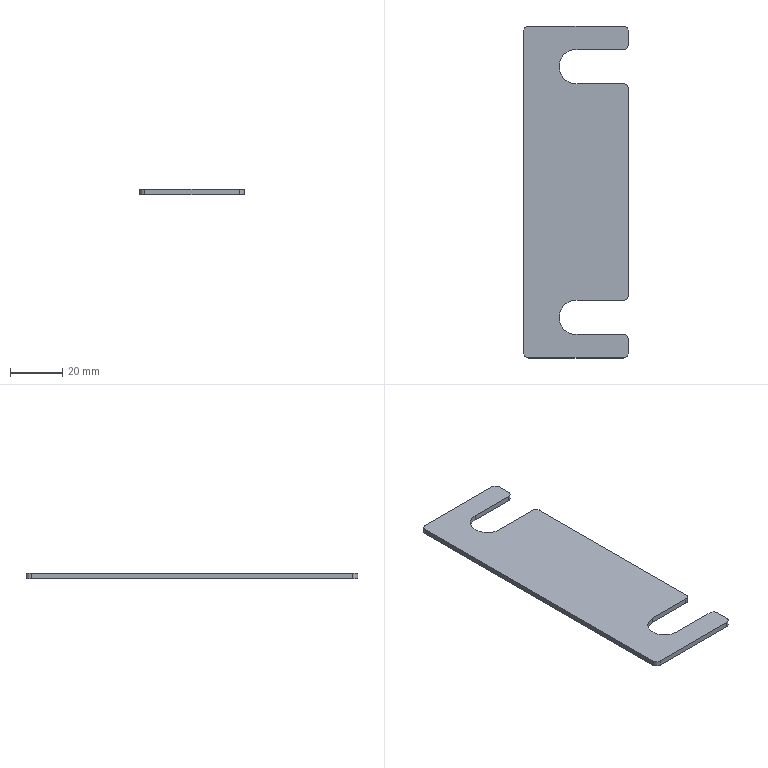Part | SolidWorks | features ICE 2, Extrusion 1, Fillet 1 | 1 solid | 22 faces | box 40 x 127 x 2 mm | volume 8841 mm3 | plane 12 | cylinder 10 | commonest cylinder face diameters 4 x8 13 x2
STEP:
#1=CARTESIAN_POINT('',(20.,56.5,2.));
#2=VERTEX_POINT('',#1);
#3=CARTESIAN_POINT('',(20.,61.5,2.));
#4=VERTEX_POINT('',#3);
#5=CARTESIAN_POINT('',(20.,-63.5,2.));
#6=DIRECTION('',(0.,1.,0.));
#7=VECTOR('',#6,1000.);
#8=LINE('',#5,#7);
#9=EDGE_CURVE('',#2,#4,#8,.T.);
#10=ORIENTED_EDGE('',*,*,#9,.F.);
#11=CARTESIAN_POINT('',(20.,56.5,0.));
#12=VERTEX_POINT('',#11);
#13=CARTESIAN_POINT('',(20.,56.5,2.));
#14=DIRECTION('',(0.,0.,-1.));
#15=VECTOR('',#14,1000.);
#16=LINE('',#13,#15);
#17=EDGE_CURVE('',#2,#12,#16,.T.);
#18=ORIENTED_EDGE('',*,*,#17,.T.);
#19=CARTESIAN_POINT('',(20.,61.5,0.));
#20=VERTEX_POINT('',#19);
#21=CARTESIAN_POINT('',(20.,-63.5,0.));
#22=DIRECTION('',(0.,1.,0.));
#23=VECTOR('',#22,1000.);
#24=LINE('',#21,#23);
#25=EDGE_CURVE('',#12,#20,#24,.T.);
#26=ORIENTED_EDGE('',*,*,#25,.T.);
#27=CARTESIAN_POINT('',(20.,61.5,2.));
#28=DIRECTION('',(0.,0.,1.));
#29=VECTOR('',#28,1000.);
#30=LINE('',#27,#29);
#31=EDGE_CURVE('',#20,#4,#30,.T.);
#32=ORIENTED_EDGE('',*,*,#31,.T.);
#33=EDGE_LOOP('',(#10,#18,#26,#32));
#34=FACE_OUTER_BOUND('',#33,.T.);
#35=CARTESIAN_POINT('',(20.,-63.5,2.));
#36=DIRECTION('',(-1.,0.,0.));
#37=DIRECTION('',(0.,-1.,0.));
#38=AXIS2_PLACEMENT_3D('',#35,#36,#37);
#39=PLANE('',#38);
#40=ADVANCED_FACE('',(#34),#39,.F.);
#41=CARTESIAN_POINT('',(20.,-39.5,2.));
#42=VERTEX_POINT('',#41);
#43=CARTESIAN_POINT('',(20.,39.5,2.));
#44=VERTEX_POINT('',#43);
#45=CARTESIAN_POINT('',(20.,-63.5,2.));
#46=DIRECTION('',(0.,1.,0.));
#47=VECTOR('',#46,1000.);
#48=LINE('',#45,#47);
#49=EDGE_CURVE('',#42,#44,#48,.T.);
#50=ORIENTED_EDGE('',*,*,#49,.F.);
#51=CARTESIAN_POINT('',(20.,-39.5,0.));
#52=VERTEX_POINT('',#51);
#53=CARTESIAN_POINT('',(20.,-39.5,2.));
#54=DIRECTION('',(0.,0.,-1.));
#55=VECTOR('',#54,1000.);
#56=LINE('',#53,#55);
#57=EDGE_CURVE('',#42,#52,#56,.T.);
#58=ORIENTED_EDGE('',*,*,#57,.T.);
#59=CARTESIAN_POINT('',(20.,39.5,0.));
#60=VERTEX_POINT('',#59);
#61=CARTESIAN_POINT('',(20.,-63.5,0.));
#62=DIRECTION('',(0.,1.,0.));
#63=VECTOR('',#62,1000.);
#64=LINE('',#61,#63);
#65=EDGE_CURVE('',#52,#60,#64,.T.);
#66=ORIENTED_EDGE('',*,*,#65,.T.);
#67=CARTESIAN_POINT('',(20.,39.5,2.));
#68=DIRECTION('',(0.,0.,1.));
#69=VECTOR('',#68,1000.);
#70=LINE('',#67,#69);
#71=EDGE_CURVE('',#60,#44,#70,.T.);
#72=ORIENTED_EDGE('',*,*,#71,.T.);
#73=EDGE_LOOP('',(#50,#58,#66,#72));
#74=FACE_OUTER_BOUND('',#73,.T.);
#75=CARTESIAN_POINT('',(20.,-63.5,2.));
#76=DIRECTION('',(-1.,0.,0.));
#77=DIRECTION('',(0.,-1.,0.));
#78=AXIS2_PLACEMENT_3D('',#75,#76,#77);
#79=PLANE('',#78);
#80=ADVANCED_FACE('',(#74),#79,.F.);
#81=CARTESIAN_POINT('',(0.,-41.5,2.));
#82=VERTEX_POINT('',#81);
#83=CARTESIAN_POINT('',(0.,-41.5,0.));
#84=VERTEX_POINT('',#83);
#85=CARTESIAN_POINT('',(0.,-41.5,-1.));
#86=DIRECTION('',(0.,0.,-1.));
#87=VECTOR('',#86,1000.);
#88=LINE('',#85,#87);
#89=EDGE_CURVE('',#82,#84,#88,.T.);
#90=ORIENTED_EDGE('',*,*,#89,.F.);
#91=CARTESIAN_POINT('',(0.,-54.5,2.));
#92=VERTEX_POINT('',#91);
#93=CARTESIAN_POINT('',(0.,-48.,2.));
#94=DIRECTION('',(0.,0.,1.));
#95=DIRECTION('',(1.,0.,0.));
#96=AXIS2_PLACEMENT_3D('',#93,#94,#95);
#97=CIRCLE('',#96,6.5);
#98=EDGE_CURVE('',#82,#92,#97,.T.);
#99=ORIENTED_EDGE('',*,*,#98,.T.);
#100=CARTESIAN_POINT('',(0.,-54.5,0.));
#101=VERTEX_POINT('',#100);
#102=CARTESIAN_POINT('',(0.,-54.5,-1.));
#103=DIRECTION('',(0.,0.,-1.));
#104=VECTOR('',#103,1000.);
#105=LINE('',#102,#104);
#106=EDGE_CURVE('',#92,#101,#105,.T.);
#107=ORIENTED_EDGE('',*,*,#106,.T.);
#108=CARTESIAN_POINT('',(0.,-48.,0.));
#109=DIRECTION('',(0.,0.,1.));
#110=DIRECTION('',(1.,0.,0.));
#111=AXIS2_PLACEMENT_3D('',#108,#109,#110);
#112=CIRCLE('',#111,6.5);
#113=EDGE_CURVE('',#84,#101,#112,.T.);
#114=ORIENTED_EDGE('',*,*,#113,.F.);
#115=EDGE_LOOP('',(#90,#99,#107,#114));
#116=FACE_OUTER_BOUND('',#115,.T.);
#117=CARTESIAN_POINT('',(0.,-48.,-1.));
#118=DIRECTION('',(0.,0.,1.));
#119=DIRECTION('',(1.,0.,0.));
#120=AXIS2_PLACEMENT_3D('',#117,#118,#119);
#121=CYLINDRICAL_SURFACE('',#120,6.5);
#122=ADVANCED_FACE('',(#116),#121,.F.);
#123=CARTESIAN_POINT('',(0.,54.5,2.));
#124=VERTEX_POINT('',#123);
#125=CARTESIAN_POINT('',(0.,54.5,0.));
#126=VERTEX_POINT('',#125);
#127=CARTESIAN_POINT('',(0.,54.5,-1.));
#128=DIRECTION('',(0.,0.,-1.));
#129=VECTOR('',#128,1000.);
#130=LINE('',#127,#129);
#131=EDGE_CURVE('',#124,#126,#130,.T.);
#132=ORIENTED_EDGE('',*,*,#131,.F.);
#133=CARTESIAN_POINT('',(0.,41.5,2.));
#134=VERTEX_POINT('',#133);
#135=CARTESIAN_POINT('',(0.,48.,2.));
#136=DIRECTION('',(0.,0.,1.));
#137=DIRECTION('',(1.,0.,0.));
#138=AXIS2_PLACEMENT_3D('',#135,#136,#137);
#139=CIRCLE('',#138,6.5);
#140=EDGE_CURVE('',#124,#134,#139,.T.);
#141=ORIENTED_EDGE('',*,*,#140,.T.);
#142=CARTESIAN_POINT('',(0.,41.5,0.));
#143=VERTEX_POINT('',#142);
#144=CARTESIAN_POINT('',(0.,41.5,-1.));
#145=DIRECTION('',(0.,0.,-1.));
#146=VECTOR('',#145,1000.);
#147=LINE('',#144,#146);
#148=EDGE_CURVE('',#134,#143,#147,.T.);
#149=ORIENTED_EDGE('',*,*,#148,.T.);
#150=CARTESIAN_POINT('',(0.,48.,0.));
#151=DIRECTION('',(0.,0.,1.));
#152=DIRECTION('',(1.,0.,0.));
#153=AXIS2_PLACEMENT_3D('',#150,#151,#152);
#154=CIRCLE('',#153,6.5);
#155=EDGE_CURVE('',#126,#143,#154,.T.);
#156=ORIENTED_EDGE('',*,*,#155,.F.);
#157=EDGE_LOOP('',(#132,#141,#149,#156));
#158=FACE_OUTER_BOUND('',#157,.T.);
#159=CARTESIAN_POINT('',(0.,48.,-1.));
#160=DIRECTION('',(0.,0.,1.));
#161=DIRECTION('',(1.,0.,0.));
#162=AXIS2_PLACEMENT_3D('',#159,#160,#161);
#163=CYLINDRICAL_SURFACE('',#162,6.5);
#164=ADVANCED_FACE('',(#158),#163,.F.);
#165=CARTESIAN_POINT('',(-20.,61.5,0.));
#166=VERTEX_POINT('',#165);
#167=CARTESIAN_POINT('',(-20.,-61.5,0.));
#168=VERTEX_POINT('',#167);
#169=CARTESIAN_POINT('',(-20.,-63.5,0.));
#170=DIRECTION('',(0.,-1.,0.));
#171=VECTOR('',#170,1000.);
#172=LINE('',#169,#171);
#173=EDGE_CURVE('',#166,#168,#172,.T.);
#174=ORIENTED_EDGE('',*,*,#173,.T.);
#175=CARTESIAN_POINT('',(-20.,-61.5,2.));
#176=VERTEX_POINT('',#175);
#177=CARTESIAN_POINT('',(-20.,-61.5,2.));
#178=DIRECTION('',(0.,0.,1.));
#179=VECTOR('',#178,1000.);
#180=LINE('',#177,#179);
#181=EDGE_CURVE('',#168,#176,#180,.T.);
#182=ORIENTED_EDGE('',*,*,#181,.T.);
#183=CARTESIAN_POINT('',(-20.,61.5,2.));
#184=VERTEX_POINT('',#183);
#185=CARTESIAN_POINT('',(-20.,-63.5,2.));
#186=DIRECTION('',(0.,-1.,0.));
#187=VECTOR('',#186,1000.);
#188=LINE('',#185,#187);
#189=EDGE_CURVE('',#184,#176,#188,.T.);
#190=ORIENTED_EDGE('',*,*,#189,.F.);
#191=CARTESIAN_POINT('',(-20.,61.5,2.));
#192=DIRECTION('',(0.,0.,-1.));
#193=VECTOR('',#192,1000.);
#194=LINE('',#191,#193);
#195=EDGE_CURVE('',#184,#166,#194,.T.);
#196=ORIENTED_EDGE('',*,*,#195,.T.);
#197=EDGE_LOOP('',(#174,#182,#190,#196));
#198=FACE_OUTER_BOUND('',#197,.T.);
#199=CARTESIAN_POINT('',(-20.,-63.5,2.));
#200=DIRECTION('',(1.,0.,0.));
#201=DIRECTION('',(0.,0.,-1.));
#202=AXIS2_PLACEMENT_3D('',#199,#200,#201);
#203=PLANE('',#202);
#204=ADVANCED_FACE('',(#198),#203,.F.);
#205=CARTESIAN_POINT('',(-18.,-63.5,2.));
#206=VERTEX_POINT('',#205);
#207=CARTESIAN_POINT('',(18.,-63.5,2.));
#208=VERTEX_POINT('',#207);
#209=CARTESIAN_POINT('',(20.,-63.5,2.));
#210=DIRECTION('',(1.,0.,0.));
#211=VECTOR('',#210,1000.);
#212=LINE('',#209,#211);
#213=EDGE_CURVE('',#206,#208,#212,.T.);
#214=ORIENTED_EDGE('',*,*,#213,.F.);
#215=CARTESIAN_POINT('',(-18.,-63.5,0.));
#216=VERTEX_POINT('',#215);
#217=CARTESIAN_POINT('',(-18.,-63.5,2.));
#218=DIRECTION('',(0.,0.,-1.));
#219=VECTOR('',#218,1000.);
#220=LINE('',#217,#219);
#221=EDGE_CURVE('',#206,#216,#220,.T.);
#222=ORIENTED_EDGE('',*,*,#221,.T.);
#223=CARTESIAN_POINT('',(18.,-63.5,0.));
#224=VERTEX_POINT('',#223);
#225=CARTESIAN_POINT('',(20.,-63.5,0.));
#226=DIRECTION('',(1.,0.,0.));
#227=VECTOR('',#226,1000.);
#228=LINE('',#225,#227);
#229=EDGE_CURVE('',#216,#224,#228,.T.);
#230=ORIENTED_EDGE('',*,*,#229,.T.);
#231=CARTESIAN_POINT('',(18.,-63.5,2.));
#232=DIRECTION('',(0.,0.,1.));
#233=VECTOR('',#232,1000.);
#234=LINE('',#231,#233);
#235=EDGE_CURVE('',#224,#208,#234,.T.);
#236=ORIENTED_EDGE('',*,*,#235,.T.);
#237=EDGE_LOOP('',(#214,#222,#230,#236));
#238=FACE_OUTER_BOUND('',#237,.T.);
#239=CARTESIAN_POINT('',(20.,-63.5,2.));
#240=DIRECTION('',(0.,1.,0.));
#241=DIRECTION('',(-1.,0.,0.));
#242=AXIS2_PLACEMENT_3D('',#239,#240,#241);
#243=PLANE('',#242);
#244=ADVANCED_FACE('',(#238),#243,.F.);
#245=CARTESIAN_POINT('',(20.,-61.5,0.));
#246=VERTEX_POINT('',#245);
#247=CARTESIAN_POINT('',(20.,-56.5,0.));
#248=VERTEX_POINT('',#247);
#249=CARTESIAN_POINT('',(20.,-63.5,0.));
#250=DIRECTION('',(0.,1.,0.));
#251=VECTOR('',#250,1000.);
#252=LINE('',#249,#251);
#253=EDGE_CURVE('',#246,#248,#252,.T.);
#254=ORIENTED_EDGE('',*,*,#253,.T.);
#255=CARTESIAN_POINT('',(20.,-56.5,2.));
#256=VERTEX_POINT('',#255);
#257=CARTESIAN_POINT('',(20.,-56.5,2.));
#258=DIRECTION('',(0.,0.,1.));
#259=VECTOR('',#258,1000.);
#260=LINE('',#257,#259);
#261=EDGE_CURVE('',#248,#256,#260,.T.);
#262=ORIENTED_EDGE('',*,*,#261,.T.);
#263=CARTESIAN_POINT('',(20.,-61.5,2.));
#264=VERTEX_POINT('',#263);
#265=CARTESIAN_POINT('',(20.,-63.5,2.));
#266=DIRECTION('',(0.,1.,0.));
#267=VECTOR('',#266,1000.);
#268=LINE('',#265,#267);
#269=EDGE_CURVE('',#264,#256,#268,.T.);
#270=ORIENTED_EDGE('',*,*,#269,.F.);
#271=CARTESIAN_POINT('',(20.,-61.5,2.));
#272=DIRECTION('',(0.,0.,-1.));
#273=VECTOR('',#272,1000.);
#274=LINE('',#271,#273);
#275=EDGE_CURVE('',#264,#246,#274,.T.);
#276=ORIENTED_EDGE('',*,*,#275,.T.);
#277=EDGE_LOOP('',(#254,#262,#270,#276));
#278=FACE_OUTER_BOUND('',#277,.T.);
#279=CARTESIAN_POINT('',(20.,-63.5,2.));
#280=DIRECTION('',(-1.,0.,0.));
#281=DIRECTION('',(0.,-1.,0.));
#282=AXIS2_PLACEMENT_3D('',#279,#280,#281);
#283=PLANE('',#282);
#284=ADVANCED_FACE('',(#278),#283,.F.);
#285=CARTESIAN_POINT('',(18.,63.5,0.));
#286=VERTEX_POINT('',#285);
#287=CARTESIAN_POINT('',(-18.,63.5,0.));
#288=VERTEX_POINT('',#287);
#289=CARTESIAN_POINT('',(20.,63.5,0.));
#290=DIRECTION('',(-1.,0.,0.));
#291=VECTOR('',#290,1000.);
#292=LINE('',#289,#291);
#293=EDGE_CURVE('',#286,#288,#292,.T.);
#294=ORIENTED_EDGE('',*,*,#293,.T.);
#295=CARTESIAN_POINT('',(-18.,63.5,2.));
#296=VERTEX_POINT('',#295);
#297=CARTESIAN_POINT('',(-18.,63.5,2.));
#298=DIRECTION('',(0.,0.,1.));
#299=VECTOR('',#298,1000.);
#300=LINE('',#297,#299);
#301=EDGE_CURVE('',#288,#296,#300,.T.);
#302=ORIENTED_EDGE('',*,*,#301,.T.);
#303=CARTESIAN_POINT('',(18.,63.5,2.));
#304=VERTEX_POINT('',#303);
#305=CARTESIAN_POINT('',(20.,63.5,2.));
#306=DIRECTION('',(-1.,0.,0.));
#307=VECTOR('',#306,1000.);
#308=LINE('',#305,#307);
#309=EDGE_CURVE('',#304,#296,#308,.T.);
#310=ORIENTED_EDGE('',*,*,#309,.F.);
#311=CARTESIAN_POINT('',(18.,63.5,2.));
#312=DIRECTION('',(0.,0.,-1.));
#313=VECTOR('',#312,1000.);
#314=LINE('',#311,#313);
#315=EDGE_CURVE('',#304,#286,#314,.T.);
#316=ORIENTED_EDGE('',*,*,#315,.T.);
#317=EDGE_LOOP('',(#294,#302,#310,#316));
#318=FACE_OUTER_BOUND('',#317,.T.);
#319=CARTESIAN_POINT('',(20.,63.5,2.));
#320=DIRECTION('',(0.,-1.,0.));
#321=DIRECTION('',(0.,0.,-1.));
#322=AXIS2_PLACEMENT_3D('',#319,#320,#321);
#323=PLANE('',#322);
#324=ADVANCED_FACE('',(#318),#323,.F.);
#325=ORIENTED_EDGE('',*,*,#269,.T.);
#326=CARTESIAN_POINT('',(18.,-54.5,2.));
#327=VERTEX_POINT('',#326);
#328=CARTESIAN_POINT('',(18.,-56.5,2.));
#329=DIRECTION('',(0.,0.,1.));
#330=DIRECTION('',(1.,0.,0.));
#331=AXIS2_PLACEMENT_3D('',#328,#329,#330);
#332=CIRCLE('',#331,2.);
#333=EDGE_CURVE('',#256,#327,#332,.T.);
#334=ORIENTED_EDGE('',*,*,#333,.T.);
#335=CARTESIAN_POINT('',(0.,-54.5,2.));
#336=DIRECTION('',(1.,0.,0.));
#337=VECTOR('',#336,1000.);
#338=LINE('',#335,#337);
#339=EDGE_CURVE('',#92,#327,#338,.T.);
#340=ORIENTED_EDGE('',*,*,#339,.F.);
#341=ORIENTED_EDGE('',*,*,#98,.F.);
#342=CARTESIAN_POINT('',(18.,-41.5,2.));
#343=VERTEX_POINT('',#342);
#344=CARTESIAN_POINT('',(0.,-41.5,2.));
#345=DIRECTION('',(-1.,0.,0.));
#346=VECTOR('',#345,1000.);
#347=LINE('',#344,#346);
#348=EDGE_CURVE('',#343,#82,#347,.T.);
#349=ORIENTED_EDGE('',*,*,#348,.F.);
#350=CARTESIAN_POINT('',(18.,-39.5,2.));
#351=DIRECTION('',(0.,0.,1.));
#352=DIRECTION('',(1.,0.,0.));
#353=AXIS2_PLACEMENT_3D('',#350,#351,#352);
#354=CIRCLE('',#353,2.);
#355=EDGE_CURVE('',#343,#42,#354,.T.);
#356=ORIENTED_EDGE('',*,*,#355,.T.);
#357=ORIENTED_EDGE('',*,*,#49,.T.);
#358=CARTESIAN_POINT('',(18.,41.5,2.));
#359=VERTEX_POINT('',#358);
#360=CARTESIAN_POINT('',(18.,39.5,2.));
#361=DIRECTION('',(0.,0.,1.));
#362=DIRECTION('',(1.,0.,0.));
#363=AXIS2_PLACEMENT_3D('',#360,#361,#362);
#364=CIRCLE('',#363,2.);
#365=EDGE_CURVE('',#44,#359,#364,.T.);
#366=ORIENTED_EDGE('',*,*,#365,.T.);
#367=CARTESIAN_POINT('',(0.,41.5,2.));
#368=DIRECTION('',(1.,0.,0.));
#369=VECTOR('',#368,1000.);
#370=LINE('',#367,#369);
#371=EDGE_CURVE('',#134,#359,#370,.T.);
#372=ORIENTED_EDGE('',*,*,#371,.F.);
#373=ORIENTED_EDGE('',*,*,#140,.F.);
#374=CARTESIAN_POINT('',(18.,54.5,2.));
#375=VERTEX_POINT('',#374);
#376=CARTESIAN_POINT('',(0.,54.5,2.));
#377=DIRECTION('',(-1.,0.,0.));
#378=VECTOR('',#377,1000.);
#379=LINE('',#376,#378);
#380=EDGE_CURVE('',#375,#124,#379,.T.);
#381=ORIENTED_EDGE('',*,*,#380,.F.);
#382=CARTESIAN_POINT('',(18.,56.5,2.));
#383=DIRECTION('',(0.,0.,1.));
#384=DIRECTION('',(1.,0.,0.));
#385=AXIS2_PLACEMENT_3D('',#382,#383,#384);
#386=CIRCLE('',#385,2.);
#387=EDGE_CURVE('',#375,#2,#386,.T.);
#388=ORIENTED_EDGE('',*,*,#387,.T.);
#389=ORIENTED_EDGE('',*,*,#9,.T.);
#390=CARTESIAN_POINT('',(18.,61.5,2.));
#391=DIRECTION('',(0.,0.,1.));
#392=DIRECTION('',(1.,0.,0.));
#393=AXIS2_PLACEMENT_3D('',#390,#391,#392);
#394=CIRCLE('',#393,2.);
#395=EDGE_CURVE('',#4,#304,#394,.T.);
#396=ORIENTED_EDGE('',*,*,#395,.T.);
#397=ORIENTED_EDGE('',*,*,#309,.T.);
#398=CARTESIAN_POINT('',(-18.,61.5,2.));
#399=DIRECTION('',(0.,0.,1.));
#400=DIRECTION('',(1.,0.,0.));
#401=AXIS2_PLACEMENT_3D('',#398,#399,#400);
#402=CIRCLE('',#401,2.);
#403=EDGE_CURVE('',#296,#184,#402,.T.);
#404=ORIENTED_EDGE('',*,*,#403,.T.);
#405=ORIENTED_EDGE('',*,*,#189,.T.);
#406=CARTESIAN_POINT('',(-18.,-61.5,2.));
#407=DIRECTION('',(0.,0.,1.));
#408=DIRECTION('',(1.,0.,0.));
#409=AXIS2_PLACEMENT_3D('',#406,#407,#408);
#410=CIRCLE('',#409,2.);
#411=EDGE_CURVE('',#176,#206,#410,.T.);
#412=ORIENTED_EDGE('',*,*,#411,.T.);
#413=ORIENTED_EDGE('',*,*,#213,.T.);
#414=CARTESIAN_POINT('',(18.,-61.5,2.));
#415=DIRECTION('',(0.,0.,1.));
#416=DIRECTION('',(1.,0.,0.));
#417=AXIS2_PLACEMENT_3D('',#414,#415,#416);
#418=CIRCLE('',#417,2.);
#419=EDGE_CURVE('',#208,#264,#418,.T.);
#420=ORIENTED_EDGE('',*,*,#419,.T.);
#421=EDGE_LOOP('',(#325,#334,#340,#341,#349,#356,#357,#366,#372,#373,#381,#388,#389,#396,#397,#404,#405,#412,#413,#420));
#422=FACE_OUTER_BOUND('',#421,.T.);
#423=CARTESIAN_POINT('',(0.,0.,2.));
#424=DIRECTION('',(0.,0.,1.));
#425=DIRECTION('',(1.,0.,0.));
#426=AXIS2_PLACEMENT_3D('',#423,#424,#425);
#427=PLANE('',#426);
#428=ADVANCED_FACE('',(#422),#427,.T.);
#429=CARTESIAN_POINT('',(18.,-54.5,0.));
#430=VERTEX_POINT('',#429);
#431=CARTESIAN_POINT('',(0.,-54.5,0.));
#432=DIRECTION('',(1.,0.,0.));
#433=VECTOR('',#432,1000.);
#434=LINE('',#431,#433);
#435=EDGE_CURVE('',#101,#430,#434,.T.);
#436=ORIENTED_EDGE('',*,*,#435,.T.);
#437=CARTESIAN_POINT('',(18.,-56.5,0.));
#438=DIRECTION('',(0.,0.,-1.));
#439=DIRECTION('',(1.,0.,0.));
#440=AXIS2_PLACEMENT_3D('',#437,#438,#439);
#441=CIRCLE('',#440,2.);
#442=EDGE_CURVE('',#430,#248,#441,.T.);
#443=ORIENTED_EDGE('',*,*,#442,.T.);
#444=ORIENTED_EDGE('',*,*,#253,.F.);
#445=CARTESIAN_POINT('',(18.,-61.5,0.));
#446=DIRECTION('',(0.,0.,-1.));
#447=DIRECTION('',(1.,0.,0.));
#448=AXIS2_PLACEMENT_3D('',#445,#446,#447);
#449=CIRCLE('',#448,2.);
#450=EDGE_CURVE('',#246,#224,#449,.T.);
#451=ORIENTED_EDGE('',*,*,#450,.T.);
#452=ORIENTED_EDGE('',*,*,#229,.F.);
#453=CARTESIAN_POINT('',(-18.,-61.5,0.));
#454=DIRECTION('',(0.,0.,-1.));
#455=DIRECTION('',(1.,0.,0.));
#456=AXIS2_PLACEMENT_3D('',#453,#454,#455);
#457=CIRCLE('',#456,2.);
#458=EDGE_CURVE('',#216,#168,#457,.T.);
#459=ORIENTED_EDGE('',*,*,#458,.T.);
#460=ORIENTED_EDGE('',*,*,#173,.F.);
#461=CARTESIAN_POINT('',(-18.,61.5,0.));
#462=DIRECTION('',(0.,0.,-1.));
#463=DIRECTION('',(1.,0.,0.));
#464=AXIS2_PLACEMENT_3D('',#461,#462,#463);
#465=CIRCLE('',#464,2.);
#466=EDGE_CURVE('',#166,#288,#465,.T.);
#467=ORIENTED_EDGE('',*,*,#466,.T.);
#468=ORIENTED_EDGE('',*,*,#293,.F.);
#469=CARTESIAN_POINT('',(18.,61.5,0.));
#470=DIRECTION('',(0.,0.,-1.));
#471=DIRECTION('',(1.,0.,0.));
#472=AXIS2_PLACEMENT_3D('',#469,#470,#471);
#473=CIRCLE('',#472,2.);
#474=EDGE_CURVE('',#286,#20,#473,.T.);
#475=ORIENTED_EDGE('',*,*,#474,.T.);
#476=ORIENTED_EDGE('',*,*,#25,.F.);
#477=CARTESIAN_POINT('',(18.,54.5,0.));
#478=VERTEX_POINT('',#477);
#479=CARTESIAN_POINT('',(18.,56.5,0.));
#480=DIRECTION('',(0.,0.,-1.));
#481=DIRECTION('',(1.,0.,0.));
#482=AXIS2_PLACEMENT_3D('',#479,#480,#481);
#483=CIRCLE('',#482,2.);
#484=EDGE_CURVE('',#12,#478,#483,.T.);
#485=ORIENTED_EDGE('',*,*,#484,.T.);
#486=CARTESIAN_POINT('',(0.,54.5,0.));
#487=DIRECTION('',(-1.,0.,0.));
#488=VECTOR('',#487,1000.);
#489=LINE('',#486,#488);
#490=EDGE_CURVE('',#478,#126,#489,.T.);
#491=ORIENTED_EDGE('',*,*,#490,.T.);
#492=ORIENTED_EDGE('',*,*,#155,.T.);
#493=CARTESIAN_POINT('',(18.,41.5,0.));
#494=VERTEX_POINT('',#493);
#495=CARTESIAN_POINT('',(0.,41.5,0.));
#496=DIRECTION('',(1.,0.,0.));
#497=VECTOR('',#496,1000.);
#498=LINE('',#495,#497);
#499=EDGE_CURVE('',#143,#494,#498,.T.);
#500=ORIENTED_EDGE('',*,*,#499,.T.);
#501=CARTESIAN_POINT('',(18.,39.5,0.));
#502=DIRECTION('',(0.,0.,-1.));
#503=DIRECTION('',(1.,0.,0.));
#504=AXIS2_PLACEMENT_3D('',#501,#502,#503);
#505=CIRCLE('',#504,2.);
#506=EDGE_CURVE('',#494,#60,#505,.T.);
#507=ORIENTED_EDGE('',*,*,#506,.T.);
#508=ORIENTED_EDGE('',*,*,#65,.F.);
#509=CARTESIAN_POINT('',(18.,-41.5,0.));
#510=VERTEX_POINT('',#509);
#511=CARTESIAN_POINT('',(18.,-39.5,0.));
#512=DIRECTION('',(0.,0.,-1.));
#513=DIRECTION('',(1.,0.,0.));
#514=AXIS2_PLACEMENT_3D('',#511,#512,#513);
#515=CIRCLE('',#514,2.);
#516=EDGE_CURVE('',#52,#510,#515,.T.);
#517=ORIENTED_EDGE('',*,*,#516,.T.);
#518=CARTESIAN_POINT('',(0.,-41.5,0.));
#519=DIRECTION('',(-1.,0.,0.));
#520=VECTOR('',#519,1000.);
#521=LINE('',#518,#520);
#522=EDGE_CURVE('',#510,#84,#521,.T.);
#523=ORIENTED_EDGE('',*,*,#522,.T.);
#524=ORIENTED_EDGE('',*,*,#113,.T.);
#525=EDGE_LOOP('',(#436,#443,#444,#451,#452,#459,#460,#467,#468,#475,#476,#485,#491,#492,#500,#507,#508,#517,#523,#524));
#526=FACE_OUTER_BOUND('',#525,.T.);
#527=CARTESIAN_POINT('',(0.,0.,0.));
#528=DIRECTION('',(0.,0.,1.));
#529=DIRECTION('',(1.,0.,0.));
#530=AXIS2_PLACEMENT_3D('',#527,#528,#529);
#531=PLANE('',#530);
#532=ADVANCED_FACE('',(#526),#531,.F.);
#533=ORIENTED_EDGE('',*,*,#371,.T.);
#534=CARTESIAN_POINT('',(18.,41.5,-8.));
#535=DIRECTION('',(0.,0.,-1.));
#536=VECTOR('',#535,1000.);
#537=LINE('',#534,#536);
#538=EDGE_CURVE('',#359,#494,#537,.T.);
#539=ORIENTED_EDGE('',*,*,#538,.T.);
#540=ORIENTED_EDGE('',*,*,#499,.F.);
#541=ORIENTED_EDGE('',*,*,#148,.F.);
#542=EDGE_LOOP('',(#533,#539,#540,#541));
#543=FACE_OUTER_BOUND('',#542,.T.);
#544=CARTESIAN_POINT('',(0.,41.5,-8.));
#545=DIRECTION('',(0.,-1.,0.));
#546=DIRECTION('',(0.,0.,-1.));
#547=AXIS2_PLACEMENT_3D('',#544,#545,#546);
#548=PLANE('',#547);
#549=ADVANCED_FACE('',(#543),#548,.F.);
#550=ORIENTED_EDGE('',*,*,#490,.F.);
#551=CARTESIAN_POINT('',(18.,54.5,-8.));
#552=DIRECTION('',(0.,0.,1.));
#553=VECTOR('',#552,1000.);
#554=LINE('',#551,#553);
#555=EDGE_CURVE('',#478,#375,#554,.T.);
#556=ORIENTED_EDGE('',*,*,#555,.T.);
#557=ORIENTED_EDGE('',*,*,#380,.T.);
#558=ORIENTED_EDGE('',*,*,#131,.T.);
#559=EDGE_LOOP('',(#550,#556,#557,#558));
#560=FACE_OUTER_BOUND('',#559,.T.);
#561=CARTESIAN_POINT('',(0.,54.5,-8.));
#562=DIRECTION('',(0.,1.,0.));
#563=DIRECTION('',(-1.,0.,0.));
#564=AXIS2_PLACEMENT_3D('',#561,#562,#563);
#565=PLANE('',#564);
#566=ADVANCED_FACE('',(#560),#565,.F.);
#567=ORIENTED_EDGE('',*,*,#339,.T.);
#568=CARTESIAN_POINT('',(18.,-54.5,-8.));
#569=DIRECTION('',(0.,0.,-1.));
#570=VECTOR('',#569,1000.);
#571=LINE('',#568,#570);
#572=EDGE_CURVE('',#327,#430,#571,.T.);
#573=ORIENTED_EDGE('',*,*,#572,.T.);
#574=ORIENTED_EDGE('',*,*,#435,.F.);
#575=ORIENTED_EDGE('',*,*,#106,.F.);
#576=EDGE_LOOP('',(#567,#573,#574,#575));
#577=FACE_OUTER_BOUND('',#576,.T.);
#578=CARTESIAN_POINT('',(0.,-54.5,-8.));
#579=DIRECTION('',(0.,-1.,0.));
#580=DIRECTION('',(0.,0.,-1.));
#581=AXIS2_PLACEMENT_3D('',#578,#579,#580);
#582=PLANE('',#581);
#583=ADVANCED_FACE('',(#577),#582,.F.);
#584=ORIENTED_EDGE('',*,*,#522,.F.);
#585=CARTESIAN_POINT('',(18.,-41.5,-8.));
#586=DIRECTION('',(0.,0.,1.));
#587=VECTOR('',#586,1000.);
#588=LINE('',#585,#587);
#589=EDGE_CURVE('',#510,#343,#588,.T.);
#590=ORIENTED_EDGE('',*,*,#589,.T.);
#591=ORIENTED_EDGE('',*,*,#348,.T.);
#592=ORIENTED_EDGE('',*,*,#89,.T.);
#593=EDGE_LOOP('',(#584,#590,#591,#592));
#594=FACE_OUTER_BOUND('',#593,.T.);
#595=CARTESIAN_POINT('',(0.,-41.5,-8.));
#596=DIRECTION('',(0.,1.,0.));
#597=DIRECTION('',(0.,0.,1.));
#598=AXIS2_PLACEMENT_3D('',#595,#596,#597);
#599=PLANE('',#598);
#600=ADVANCED_FACE('',(#594),#599,.F.);
#601=ORIENTED_EDGE('',*,*,#442,.F.);
#602=ORIENTED_EDGE('',*,*,#572,.F.);
#603=ORIENTED_EDGE('',*,*,#333,.F.);
#604=ORIENTED_EDGE('',*,*,#261,.F.);
#605=EDGE_LOOP('',(#601,#602,#603,#604));
#606=FACE_OUTER_BOUND('',#605,.T.);
#607=CARTESIAN_POINT('',(18.,-56.5,2.));
#608=DIRECTION('',(0.,0.,1.));
#609=DIRECTION('',(1.,0.,0.));
#610=AXIS2_PLACEMENT_3D('',#607,#608,#609);
#611=CYLINDRICAL_SURFACE('',#610,2.);
#612=ADVANCED_FACE('',(#606),#611,.T.);
#613=ORIENTED_EDGE('',*,*,#516,.F.);
#614=ORIENTED_EDGE('',*,*,#57,.F.);
#615=ORIENTED_EDGE('',*,*,#355,.F.);
#616=ORIENTED_EDGE('',*,*,#589,.F.);
#617=EDGE_LOOP('',(#613,#614,#615,#616));
#618=FACE_OUTER_BOUND('',#617,.T.);
#619=CARTESIAN_POINT('',(18.,-39.5,-8.));
#620=DIRECTION('',(0.,0.,1.));
#621=DIRECTION('',(1.,0.,0.));
#622=AXIS2_PLACEMENT_3D('',#619,#620,#621);
#623=CYLINDRICAL_SURFACE('',#622,2.);
#624=ADVANCED_FACE('',(#618),#623,.T.);
#625=ORIENTED_EDGE('',*,*,#506,.F.);
#626=ORIENTED_EDGE('',*,*,#538,.F.);
#627=ORIENTED_EDGE('',*,*,#365,.F.);
#628=ORIENTED_EDGE('',*,*,#71,.F.);
#629=EDGE_LOOP('',(#625,#626,#627,#628));
#630=FACE_OUTER_BOUND('',#629,.T.);
#631=CARTESIAN_POINT('',(18.,39.5,2.));
#632=DIRECTION('',(0.,0.,1.));
#633=DIRECTION('',(1.,0.,0.));
#634=AXIS2_PLACEMENT_3D('',#631,#632,#633);
#635=CYLINDRICAL_SURFACE('',#634,2.);
#636=ADVANCED_FACE('',(#630),#635,.T.);
#637=ORIENTED_EDGE('',*,*,#484,.F.);
#638=ORIENTED_EDGE('',*,*,#17,.F.);
#639=ORIENTED_EDGE('',*,*,#387,.F.);
#640=ORIENTED_EDGE('',*,*,#555,.F.);
#641=EDGE_LOOP('',(#637,#638,#639,#640));
#642=FACE_OUTER_BOUND('',#641,.T.);
#643=CARTESIAN_POINT('',(18.,56.5,-8.));
#644=DIRECTION('',(0.,0.,1.));
#645=DIRECTION('',(1.,0.,0.));
#646=AXIS2_PLACEMENT_3D('',#643,#644,#645);
#647=CYLINDRICAL_SURFACE('',#646,2.);
#648=ADVANCED_FACE('',(#642),#647,.T.);
#649=ORIENTED_EDGE('',*,*,#411,.F.);
#650=ORIENTED_EDGE('',*,*,#181,.F.);
#651=ORIENTED_EDGE('',*,*,#458,.F.);
#652=ORIENTED_EDGE('',*,*,#221,.F.);
#653=EDGE_LOOP('',(#649,#650,#651,#652));
#654=FACE_OUTER_BOUND('',#653,.T.);
#655=CARTESIAN_POINT('',(-18.,-61.5,2.));
#656=DIRECTION('',(0.,0.,-1.));
#657=DIRECTION('',(-1.,0.,0.));
#658=AXIS2_PLACEMENT_3D('',#655,#656,#657);
#659=CYLINDRICAL_SURFACE('',#658,2.);
#660=ADVANCED_FACE('',(#654),#659,.T.);
#661=ORIENTED_EDGE('',*,*,#403,.F.);
#662=ORIENTED_EDGE('',*,*,#301,.F.);
#663=ORIENTED_EDGE('',*,*,#466,.F.);
#664=ORIENTED_EDGE('',*,*,#195,.F.);
#665=EDGE_LOOP('',(#661,#662,#663,#664));
#666=FACE_OUTER_BOUND('',#665,.T.);
#667=CARTESIAN_POINT('',(-18.,61.5,2.));
#668=DIRECTION('',(0.,0.,-1.));
#669=DIRECTION('',(-1.,0.,0.));
#670=AXIS2_PLACEMENT_3D('',#667,#668,#669);
#671=CYLINDRICAL_SURFACE('',#670,2.);
#672=ADVANCED_FACE('',(#666),#671,.T.);
#673=ORIENTED_EDGE('',*,*,#419,.F.);
#674=ORIENTED_EDGE('',*,*,#235,.F.);
#675=ORIENTED_EDGE('',*,*,#450,.F.);
#676=ORIENTED_EDGE('',*,*,#275,.F.);
#677=EDGE_LOOP('',(#673,#674,#675,#676));
#678=FACE_OUTER_BOUND('',#677,.T.);
#679=CARTESIAN_POINT('',(18.,-61.5,2.));
#680=DIRECTION('',(0.,0.,-1.));
#681=DIRECTION('',(-1.,0.,0.));
#682=AXIS2_PLACEMENT_3D('',#679,#680,#681);
#683=CYLINDRICAL_SURFACE('',#682,2.);
#684=ADVANCED_FACE('',(#678),#683,.T.);
#685=ORIENTED_EDGE('',*,*,#395,.F.);
#686=ORIENTED_EDGE('',*,*,#31,.F.);
#687=ORIENTED_EDGE('',*,*,#474,.F.);
#688=ORIENTED_EDGE('',*,*,#315,.F.);
#689=EDGE_LOOP('',(#685,#686,#687,#688));
#690=FACE_OUTER_BOUND('',#689,.T.);
#691=CARTESIAN_POINT('',(18.,61.5,2.));
#692=DIRECTION('',(0.,0.,-1.));
#693=DIRECTION('',(-1.,0.,0.));
#694=AXIS2_PLACEMENT_3D('',#691,#692,#693);
#695=CYLINDRICAL_SURFACE('',#694,2.);
#696=ADVANCED_FACE('',(#690),#695,.T.);
#697=CLOSED_SHELL('',(#40,#80,#122,#164,#204,#244,#284,#324,#428,#532,#549,#566,#583,#600,#612,#624,#636,#648,#660,#672,#684,#696));
#698=MANIFOLD_SOLID_BREP('',#697);
#699=CARTESIAN_POINT('',(0.,0.,0.));
#700=DIRECTION('',(0.,0.,1.));
#701=DIRECTION('',(1.,0.,0.));
#702=AXIS2_PLACEMENT_3D('',#699,#700,#701);
#703=(LENGTH_UNIT()NAMED_UNIT(*)SI_UNIT(.MILLI.,.METRE.));
#704=UNCERTAINTY_MEASURE_WITH_UNIT(LENGTH_MEASURE(0.00001),#703,'','');
#705=(NAMED_UNIT(*)PLANE_ANGLE_UNIT()SI_UNIT($,.RADIAN.));
#706=(NAMED_UNIT(*)SI_UNIT($,.STERADIAN.)SOLID_ANGLE_UNIT());
#707=(GEOMETRIC_REPRESENTATION_CONTEXT(3)GLOBAL_UNCERTAINTY_ASSIGNED_CONTEXT((#704))GLOBAL_UNIT_ASSIGNED_CONTEXT((#703,#705,#706))REPRESENTATION_CONTEXT('',''));
#708=ADVANCED_BREP_SHAPE_REPRESENTATION('',(#698,#702),#707);